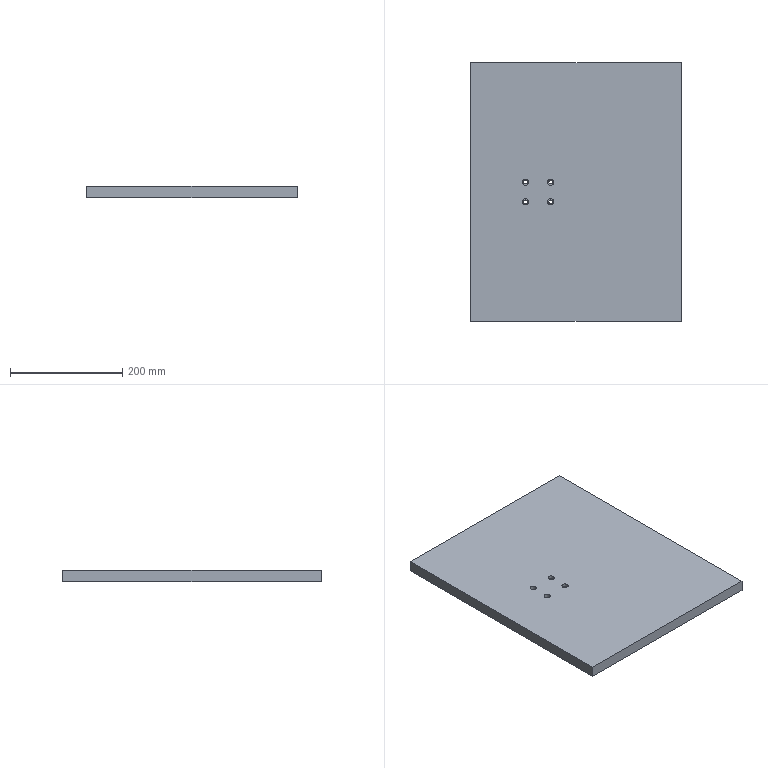Part | SolidWorks | features Extrusion 1, HoleWzd 1 | 1 solid | 26 faces | box 375 x 460 x 20 mm | volume 3445803 mm3 | cylinder 16 | plane 10 | commonest cylinder face diameters 6.6 x8 11 x8
STEP:
#1=CARTESIAN_POINT('',(-28.,247.5,14.));
#2=VERTEX_POINT('',#1);
#3=CARTESIAN_POINT('',(-17.,247.5,14.));
#4=VERTEX_POINT('',#3);
#5=CARTESIAN_POINT('',(-22.5,247.5,14.));
#6=DIRECTION('',(0.,0.,1.));
#7=DIRECTION('',(1.,0.,0.));
#8=AXIS2_PLACEMENT_3D('',#5,#6,#7);
#9=CIRCLE('',#8,5.5);
#10=EDGE_CURVE('',#2,#4,#9,.T.);
#11=ORIENTED_EDGE('',*,*,#10,.F.);
#12=CARTESIAN_POINT('',(-28.,247.5,20.));
#13=VERTEX_POINT('',#12);
#14=CARTESIAN_POINT('',(-28.,247.5,20.));
#15=DIRECTION('',(0.,0.,1.));
#16=VECTOR('',#15,1000.);
#17=LINE('',#14,#16);
#18=EDGE_CURVE('',#2,#13,#17,.T.);
#19=ORIENTED_EDGE('',*,*,#18,.T.);
#20=CARTESIAN_POINT('',(-17.,247.5,20.));
#21=VERTEX_POINT('',#20);
#22=CARTESIAN_POINT('',(-22.5,247.5,20.));
#23=DIRECTION('',(0.,0.,1.));
#24=DIRECTION('',(1.,0.,0.));
#25=AXIS2_PLACEMENT_3D('',#22,#23,#24);
#26=CIRCLE('',#25,5.5);
#27=EDGE_CURVE('',#13,#21,#26,.T.);
#28=ORIENTED_EDGE('',*,*,#27,.T.);
#29=CARTESIAN_POINT('',(-17.,247.5,20.));
#30=DIRECTION('',(0.,0.,1.));
#31=VECTOR('',#30,1000.);
#32=LINE('',#29,#31);
#33=EDGE_CURVE('',#4,#21,#32,.T.);
#34=ORIENTED_EDGE('',*,*,#33,.F.);
#35=EDGE_LOOP('',(#11,#19,#28,#34));
#36=FACE_OUTER_BOUND('',#35,.T.);
#37=CARTESIAN_POINT('',(-22.5,247.5,20.));
#38=DIRECTION('',(0.,0.,1.));
#39=DIRECTION('',(1.,0.,0.));
#40=AXIS2_PLACEMENT_3D('',#37,#38,#39);
#41=CYLINDRICAL_SURFACE('',#40,5.5);
#42=ADVANCED_FACE('',(#36),#41,.F.);
#43=CARTESIAN_POINT('',(-25.8,247.5,0.));
#44=VERTEX_POINT('',#43);
#45=CARTESIAN_POINT('',(-19.2,247.5,0.));
#46=VERTEX_POINT('',#45);
#47=CARTESIAN_POINT('',(-22.5,247.5,0.));
#48=DIRECTION('',(0.,0.,1.));
#49=DIRECTION('',(1.,0.,0.));
#50=AXIS2_PLACEMENT_3D('',#47,#48,#49);
#51=CIRCLE('',#50,3.3);
#52=EDGE_CURVE('',#44,#46,#51,.T.);
#53=ORIENTED_EDGE('',*,*,#52,.F.);
#54=CARTESIAN_POINT('',(-25.8,247.5,14.));
#55=VERTEX_POINT('',#54);
#56=CARTESIAN_POINT('',(-25.8,247.5,20.));
#57=DIRECTION('',(0.,0.,1.));
#58=VECTOR('',#57,1000.);
#59=LINE('',#56,#58);
#60=EDGE_CURVE('',#44,#55,#59,.T.);
#61=ORIENTED_EDGE('',*,*,#60,.T.);
#62=CARTESIAN_POINT('',(-19.2,247.5,14.));
#63=VERTEX_POINT('',#62);
#64=CARTESIAN_POINT('',(-22.5,247.5,14.));
#65=DIRECTION('',(0.,0.,1.));
#66=DIRECTION('',(1.,0.,0.));
#67=AXIS2_PLACEMENT_3D('',#64,#65,#66);
#68=CIRCLE('',#67,3.3);
#69=EDGE_CURVE('',#55,#63,#68,.T.);
#70=ORIENTED_EDGE('',*,*,#69,.T.);
#71=CARTESIAN_POINT('',(-19.2,247.5,20.));
#72=DIRECTION('',(0.,0.,1.));
#73=VECTOR('',#72,1000.);
#74=LINE('',#71,#73);
#75=EDGE_CURVE('',#46,#63,#74,.T.);
#76=ORIENTED_EDGE('',*,*,#75,.F.);
#77=EDGE_LOOP('',(#53,#61,#70,#76));
#78=FACE_OUTER_BOUND('',#77,.T.);
#79=CARTESIAN_POINT('',(-22.5,247.5,20.));
#80=DIRECTION('',(0.,0.,1.));
#81=DIRECTION('',(1.,0.,0.));
#82=AXIS2_PLACEMENT_3D('',#79,#80,#81);
#83=CYLINDRICAL_SURFACE('',#82,3.3);
#84=ADVANCED_FACE('',(#78),#83,.F.);
#85=CARTESIAN_POINT('',(17.,247.5,14.));
#86=VERTEX_POINT('',#85);
#87=CARTESIAN_POINT('',(28.,247.5,14.));
#88=VERTEX_POINT('',#87);
#89=CARTESIAN_POINT('',(22.5,247.5,14.));
#90=DIRECTION('',(0.,0.,1.));
#91=DIRECTION('',(1.,0.,0.));
#92=AXIS2_PLACEMENT_3D('',#89,#90,#91);
#93=CIRCLE('',#92,5.5);
#94=EDGE_CURVE('',#86,#88,#93,.T.);
#95=ORIENTED_EDGE('',*,*,#94,.F.);
#96=CARTESIAN_POINT('',(17.,247.5,20.));
#97=VERTEX_POINT('',#96);
#98=CARTESIAN_POINT('',(17.,247.5,20.));
#99=DIRECTION('',(0.,0.,1.));
#100=VECTOR('',#99,1000.);
#101=LINE('',#98,#100);
#102=EDGE_CURVE('',#86,#97,#101,.T.);
#103=ORIENTED_EDGE('',*,*,#102,.T.);
#104=CARTESIAN_POINT('',(28.,247.5,20.));
#105=VERTEX_POINT('',#104);
#106=CARTESIAN_POINT('',(22.5,247.5,20.));
#107=DIRECTION('',(0.,0.,1.));
#108=DIRECTION('',(1.,0.,0.));
#109=AXIS2_PLACEMENT_3D('',#106,#107,#108);
#110=CIRCLE('',#109,5.5);
#111=EDGE_CURVE('',#97,#105,#110,.T.);
#112=ORIENTED_EDGE('',*,*,#111,.T.);
#113=CARTESIAN_POINT('',(28.,247.5,20.));
#114=DIRECTION('',(0.,0.,1.));
#115=VECTOR('',#114,1000.);
#116=LINE('',#113,#115);
#117=EDGE_CURVE('',#88,#105,#116,.T.);
#118=ORIENTED_EDGE('',*,*,#117,.F.);
#119=EDGE_LOOP('',(#95,#103,#112,#118));
#120=FACE_OUTER_BOUND('',#119,.T.);
#121=CARTESIAN_POINT('',(22.5,247.5,20.));
#122=DIRECTION('',(0.,0.,1.));
#123=DIRECTION('',(1.,0.,0.));
#124=AXIS2_PLACEMENT_3D('',#121,#122,#123);
#125=CYLINDRICAL_SURFACE('',#124,5.5);
#126=ADVANCED_FACE('',(#120),#125,.F.);
#127=CARTESIAN_POINT('',(19.2,247.5,0.));
#128=VERTEX_POINT('',#127);
#129=CARTESIAN_POINT('',(25.8,247.5,0.));
#130=VERTEX_POINT('',#129);
#131=CARTESIAN_POINT('',(22.5,247.5,0.));
#132=DIRECTION('',(0.,0.,1.));
#133=DIRECTION('',(1.,0.,0.));
#134=AXIS2_PLACEMENT_3D('',#131,#132,#133);
#135=CIRCLE('',#134,3.3);
#136=EDGE_CURVE('',#128,#130,#135,.T.);
#137=ORIENTED_EDGE('',*,*,#136,.F.);
#138=CARTESIAN_POINT('',(19.2,247.5,14.));
#139=VERTEX_POINT('',#138);
#140=CARTESIAN_POINT('',(19.2,247.5,20.));
#141=DIRECTION('',(0.,0.,1.));
#142=VECTOR('',#141,1000.);
#143=LINE('',#140,#142);
#144=EDGE_CURVE('',#128,#139,#143,.T.);
#145=ORIENTED_EDGE('',*,*,#144,.T.);
#146=CARTESIAN_POINT('',(25.8,247.5,14.));
#147=VERTEX_POINT('',#146);
#148=CARTESIAN_POINT('',(22.5,247.5,14.));
#149=DIRECTION('',(0.,0.,1.));
#150=DIRECTION('',(1.,0.,0.));
#151=AXIS2_PLACEMENT_3D('',#148,#149,#150);
#152=CIRCLE('',#151,3.3);
#153=EDGE_CURVE('',#139,#147,#152,.T.);
#154=ORIENTED_EDGE('',*,*,#153,.T.);
#155=CARTESIAN_POINT('',(25.8,247.5,20.));
#156=DIRECTION('',(0.,0.,1.));
#157=VECTOR('',#156,1000.);
#158=LINE('',#155,#157);
#159=EDGE_CURVE('',#130,#147,#158,.T.);
#160=ORIENTED_EDGE('',*,*,#159,.F.);
#161=EDGE_LOOP('',(#137,#145,#154,#160));
#162=FACE_OUTER_BOUND('',#161,.T.);
#163=CARTESIAN_POINT('',(22.5,247.5,20.));
#164=DIRECTION('',(0.,0.,1.));
#165=DIRECTION('',(1.,0.,0.));
#166=AXIS2_PLACEMENT_3D('',#163,#164,#165);
#167=CYLINDRICAL_SURFACE('',#166,3.3);
#168=ADVANCED_FACE('',(#162),#167,.F.);
#169=CARTESIAN_POINT('',(17.,212.5,14.));
#170=VERTEX_POINT('',#169);
#171=CARTESIAN_POINT('',(28.,212.5,14.));
#172=VERTEX_POINT('',#171);
#173=CARTESIAN_POINT('',(22.5,212.5,14.));
#174=DIRECTION('',(0.,0.,1.));
#175=DIRECTION('',(1.,0.,0.));
#176=AXIS2_PLACEMENT_3D('',#173,#174,#175);
#177=CIRCLE('',#176,5.5);
#178=EDGE_CURVE('',#170,#172,#177,.T.);
#179=ORIENTED_EDGE('',*,*,#178,.F.);
#180=CARTESIAN_POINT('',(17.,212.5,20.));
#181=VERTEX_POINT('',#180);
#182=CARTESIAN_POINT('',(17.,212.5,20.));
#183=DIRECTION('',(0.,0.,1.));
#184=VECTOR('',#183,1000.);
#185=LINE('',#182,#184);
#186=EDGE_CURVE('',#170,#181,#185,.T.);
#187=ORIENTED_EDGE('',*,*,#186,.T.);
#188=CARTESIAN_POINT('',(28.,212.5,20.));
#189=VERTEX_POINT('',#188);
#190=CARTESIAN_POINT('',(22.5,212.5,20.));
#191=DIRECTION('',(0.,0.,1.));
#192=DIRECTION('',(1.,0.,0.));
#193=AXIS2_PLACEMENT_3D('',#190,#191,#192);
#194=CIRCLE('',#193,5.5);
#195=EDGE_CURVE('',#181,#189,#194,.T.);
#196=ORIENTED_EDGE('',*,*,#195,.T.);
#197=CARTESIAN_POINT('',(28.,212.5,20.));
#198=DIRECTION('',(0.,0.,1.));
#199=VECTOR('',#198,1000.);
#200=LINE('',#197,#199);
#201=EDGE_CURVE('',#172,#189,#200,.T.);
#202=ORIENTED_EDGE('',*,*,#201,.F.);
#203=EDGE_LOOP('',(#179,#187,#196,#202));
#204=FACE_OUTER_BOUND('',#203,.T.);
#205=CARTESIAN_POINT('',(22.5,212.5,20.));
#206=DIRECTION('',(0.,0.,1.));
#207=DIRECTION('',(1.,0.,0.));
#208=AXIS2_PLACEMENT_3D('',#205,#206,#207);
#209=CYLINDRICAL_SURFACE('',#208,5.5);
#210=ADVANCED_FACE('',(#204),#209,.F.);
#211=CARTESIAN_POINT('',(19.2,212.5,0.));
#212=VERTEX_POINT('',#211);
#213=CARTESIAN_POINT('',(25.8,212.5,0.));
#214=VERTEX_POINT('',#213);
#215=CARTESIAN_POINT('',(22.5,212.5,0.));
#216=DIRECTION('',(0.,0.,1.));
#217=DIRECTION('',(1.,0.,0.));
#218=AXIS2_PLACEMENT_3D('',#215,#216,#217);
#219=CIRCLE('',#218,3.3);
#220=EDGE_CURVE('',#212,#214,#219,.T.);
#221=ORIENTED_EDGE('',*,*,#220,.F.);
#222=CARTESIAN_POINT('',(19.2,212.5,14.));
#223=VERTEX_POINT('',#222);
#224=CARTESIAN_POINT('',(19.2,212.5,20.));
#225=DIRECTION('',(0.,0.,1.));
#226=VECTOR('',#225,1000.);
#227=LINE('',#224,#226);
#228=EDGE_CURVE('',#212,#223,#227,.T.);
#229=ORIENTED_EDGE('',*,*,#228,.T.);
#230=CARTESIAN_POINT('',(25.8,212.5,14.));
#231=VERTEX_POINT('',#230);
#232=CARTESIAN_POINT('',(22.5,212.5,14.));
#233=DIRECTION('',(0.,0.,1.));
#234=DIRECTION('',(1.,0.,0.));
#235=AXIS2_PLACEMENT_3D('',#232,#233,#234);
#236=CIRCLE('',#235,3.3);
#237=EDGE_CURVE('',#223,#231,#236,.T.);
#238=ORIENTED_EDGE('',*,*,#237,.T.);
#239=CARTESIAN_POINT('',(25.8,212.5,20.));
#240=DIRECTION('',(0.,0.,1.));
#241=VECTOR('',#240,1000.);
#242=LINE('',#239,#241);
#243=EDGE_CURVE('',#214,#231,#242,.T.);
#244=ORIENTED_EDGE('',*,*,#243,.F.);
#245=EDGE_LOOP('',(#221,#229,#238,#244));
#246=FACE_OUTER_BOUND('',#245,.T.);
#247=CARTESIAN_POINT('',(22.5,212.5,20.));
#248=DIRECTION('',(0.,0.,1.));
#249=DIRECTION('',(1.,0.,0.));
#250=AXIS2_PLACEMENT_3D('',#247,#248,#249);
#251=CYLINDRICAL_SURFACE('',#250,3.3);
#252=ADVANCED_FACE('',(#246),#251,.F.);
#253=CARTESIAN_POINT('',(-28.,212.5,14.));
#254=VERTEX_POINT('',#253);
#255=CARTESIAN_POINT('',(-17.,212.5,14.));
#256=VERTEX_POINT('',#255);
#257=CARTESIAN_POINT('',(-22.5,212.5,14.));
#258=DIRECTION('',(0.,0.,1.));
#259=DIRECTION('',(1.,0.,0.));
#260=AXIS2_PLACEMENT_3D('',#257,#258,#259);
#261=CIRCLE('',#260,5.5);
#262=EDGE_CURVE('',#254,#256,#261,.T.);
#263=ORIENTED_EDGE('',*,*,#262,.F.);
#264=CARTESIAN_POINT('',(-28.,212.5,20.));
#265=VERTEX_POINT('',#264);
#266=CARTESIAN_POINT('',(-28.,212.5,20.));
#267=DIRECTION('',(0.,0.,1.));
#268=VECTOR('',#267,1000.);
#269=LINE('',#266,#268);
#270=EDGE_CURVE('',#254,#265,#269,.T.);
#271=ORIENTED_EDGE('',*,*,#270,.T.);
#272=CARTESIAN_POINT('',(-17.,212.5,20.));
#273=VERTEX_POINT('',#272);
#274=CARTESIAN_POINT('',(-22.5,212.5,20.));
#275=DIRECTION('',(0.,0.,1.));
#276=DIRECTION('',(1.,0.,0.));
#277=AXIS2_PLACEMENT_3D('',#274,#275,#276);
#278=CIRCLE('',#277,5.5);
#279=EDGE_CURVE('',#265,#273,#278,.T.);
#280=ORIENTED_EDGE('',*,*,#279,.T.);
#281=CARTESIAN_POINT('',(-17.,212.5,20.));
#282=DIRECTION('',(0.,0.,1.));
#283=VECTOR('',#282,1000.);
#284=LINE('',#281,#283);
#285=EDGE_CURVE('',#256,#273,#284,.T.);
#286=ORIENTED_EDGE('',*,*,#285,.F.);
#287=EDGE_LOOP('',(#263,#271,#280,#286));
#288=FACE_OUTER_BOUND('',#287,.T.);
#289=CARTESIAN_POINT('',(-22.5,212.5,20.));
#290=DIRECTION('',(0.,0.,1.));
#291=DIRECTION('',(1.,0.,0.));
#292=AXIS2_PLACEMENT_3D('',#289,#290,#291);
#293=CYLINDRICAL_SURFACE('',#292,5.5);
#294=ADVANCED_FACE('',(#288),#293,.F.);
#295=CARTESIAN_POINT('',(-25.8,212.5,0.));
#296=VERTEX_POINT('',#295);
#297=CARTESIAN_POINT('',(-19.2,212.5,0.));
#298=VERTEX_POINT('',#297);
#299=CARTESIAN_POINT('',(-22.5,212.5,0.));
#300=DIRECTION('',(0.,0.,1.));
#301=DIRECTION('',(1.,0.,0.));
#302=AXIS2_PLACEMENT_3D('',#299,#300,#301);
#303=CIRCLE('',#302,3.3);
#304=EDGE_CURVE('',#296,#298,#303,.T.);
#305=ORIENTED_EDGE('',*,*,#304,.F.);
#306=CARTESIAN_POINT('',(-25.8,212.5,14.));
#307=VERTEX_POINT('',#306);
#308=CARTESIAN_POINT('',(-25.8,212.5,20.));
#309=DIRECTION('',(0.,0.,1.));
#310=VECTOR('',#309,1000.);
#311=LINE('',#308,#310);
#312=EDGE_CURVE('',#296,#307,#311,.T.);
#313=ORIENTED_EDGE('',*,*,#312,.T.);
#314=CARTESIAN_POINT('',(-19.2,212.5,14.));
#315=VERTEX_POINT('',#314);
#316=CARTESIAN_POINT('',(-22.5,212.5,14.));
#317=DIRECTION('',(0.,0.,1.));
#318=DIRECTION('',(1.,0.,0.));
#319=AXIS2_PLACEMENT_3D('',#316,#317,#318);
#320=CIRCLE('',#319,3.3);
#321=EDGE_CURVE('',#307,#315,#320,.T.);
#322=ORIENTED_EDGE('',*,*,#321,.T.);
#323=CARTESIAN_POINT('',(-19.2,212.5,20.));
#324=DIRECTION('',(0.,0.,1.));
#325=VECTOR('',#324,1000.);
#326=LINE('',#323,#325);
#327=EDGE_CURVE('',#298,#315,#326,.T.);
#328=ORIENTED_EDGE('',*,*,#327,.F.);
#329=EDGE_LOOP('',(#305,#313,#322,#328));
#330=FACE_OUTER_BOUND('',#329,.T.);
#331=CARTESIAN_POINT('',(-22.5,212.5,20.));
#332=DIRECTION('',(0.,0.,1.));
#333=DIRECTION('',(1.,0.,0.));
#334=AXIS2_PLACEMENT_3D('',#331,#332,#333);
#335=CYLINDRICAL_SURFACE('',#334,3.3);
#336=ADVANCED_FACE('',(#330),#335,.F.);
#337=CARTESIAN_POINT('',(-120.,460.,0.));
#338=VERTEX_POINT('',#337);
#339=CARTESIAN_POINT('',(-120.,0.,0.));
#340=VERTEX_POINT('',#339);
#341=CARTESIAN_POINT('',(-120.,460.,0.));
#342=DIRECTION('',(0.,-1.,0.));
#343=VECTOR('',#342,1000.);
#344=LINE('',#341,#343);
#345=EDGE_CURVE('',#338,#340,#344,.T.);
#346=ORIENTED_EDGE('',*,*,#345,.T.);
#347=CARTESIAN_POINT('',(-120.,0.,20.));
#348=VERTEX_POINT('',#347);
#349=CARTESIAN_POINT('',(-120.,0.,20.));
#350=DIRECTION('',(0.,0.,-1.));
#351=VECTOR('',#350,1000.);
#352=LINE('',#349,#351);
#353=EDGE_CURVE('',#348,#340,#352,.T.);
#354=ORIENTED_EDGE('',*,*,#353,.F.);
#355=CARTESIAN_POINT('',(-120.,460.,20.));
#356=VERTEX_POINT('',#355);
#357=CARTESIAN_POINT('',(-120.,460.,20.));
#358=DIRECTION('',(0.,-1.,0.));
#359=VECTOR('',#358,1000.);
#360=LINE('',#357,#359);
#361=EDGE_CURVE('',#356,#348,#360,.T.);
#362=ORIENTED_EDGE('',*,*,#361,.F.);
#363=CARTESIAN_POINT('',(-120.,460.,20.));
#364=DIRECTION('',(0.,0.,-1.));
#365=VECTOR('',#364,1000.);
#366=LINE('',#363,#365);
#367=EDGE_CURVE('',#356,#338,#366,.T.);
#368=ORIENTED_EDGE('',*,*,#367,.T.);
#369=EDGE_LOOP('',(#346,#354,#362,#368));
#370=FACE_OUTER_BOUND('',#369,.T.);
#371=CARTESIAN_POINT('',(-120.,460.,20.));
#372=DIRECTION('',(1.,0.,0.));
#373=DIRECTION('',(0.,0.,-1.));
#374=AXIS2_PLACEMENT_3D('',#371,#372,#373);
#375=PLANE('',#374);
#376=ADVANCED_FACE('',(#370),#375,.F.);
#377=CARTESIAN_POINT('',(255.,0.,0.));
#378=VERTEX_POINT('',#377);
#379=CARTESIAN_POINT('',(-120.,0.,0.));
#380=DIRECTION('',(1.,0.,0.));
#381=VECTOR('',#380,1000.);
#382=LINE('',#379,#381);
#383=EDGE_CURVE('',#340,#378,#382,.T.);
#384=ORIENTED_EDGE('',*,*,#383,.T.);
#385=CARTESIAN_POINT('',(255.,0.,20.));
#386=VERTEX_POINT('',#385);
#387=CARTESIAN_POINT('',(255.,0.,20.));
#388=DIRECTION('',(0.,0.,-1.));
#389=VECTOR('',#388,1000.);
#390=LINE('',#387,#389);
#391=EDGE_CURVE('',#386,#378,#390,.T.);
#392=ORIENTED_EDGE('',*,*,#391,.F.);
#393=CARTESIAN_POINT('',(-120.,0.,20.));
#394=DIRECTION('',(1.,0.,0.));
#395=VECTOR('',#394,1000.);
#396=LINE('',#393,#395);
#397=EDGE_CURVE('',#348,#386,#396,.T.);
#398=ORIENTED_EDGE('',*,*,#397,.F.);
#399=ORIENTED_EDGE('',*,*,#353,.T.);
#400=EDGE_LOOP('',(#384,#392,#398,#399));
#401=FACE_OUTER_BOUND('',#400,.T.);
#402=CARTESIAN_POINT('',(-120.,0.,20.));
#403=DIRECTION('',(0.,1.,0.));
#404=DIRECTION('',(-1.,0.,0.));
#405=AXIS2_PLACEMENT_3D('',#402,#403,#404);
#406=PLANE('',#405);
#407=ADVANCED_FACE('',(#401),#406,.F.);
#408=CARTESIAN_POINT('',(255.,460.,0.));
#409=VERTEX_POINT('',#408);
#410=CARTESIAN_POINT('',(255.,460.,0.));
#411=DIRECTION('',(0.,-1.,0.));
#412=VECTOR('',#411,1000.);
#413=LINE('',#410,#412);
#414=EDGE_CURVE('',#409,#378,#413,.T.);
#415=ORIENTED_EDGE('',*,*,#414,.F.);
#416=CARTESIAN_POINT('',(255.,460.,20.));
#417=VERTEX_POINT('',#416);
#418=CARTESIAN_POINT('',(255.,460.,20.));
#419=DIRECTION('',(0.,0.,-1.));
#420=VECTOR('',#419,1000.);
#421=LINE('',#418,#420);
#422=EDGE_CURVE('',#417,#409,#421,.T.);
#423=ORIENTED_EDGE('',*,*,#422,.F.);
#424=CARTESIAN_POINT('',(255.,460.,20.));
#425=DIRECTION('',(0.,-1.,0.));
#426=VECTOR('',#425,1000.);
#427=LINE('',#424,#426);
#428=EDGE_CURVE('',#417,#386,#427,.T.);
#429=ORIENTED_EDGE('',*,*,#428,.T.);
#430=ORIENTED_EDGE('',*,*,#391,.T.);
#431=EDGE_LOOP('',(#415,#423,#429,#430));
#432=FACE_OUTER_BOUND('',#431,.T.);
#433=CARTESIAN_POINT('',(255.,460.,20.));
#434=DIRECTION('',(1.,0.,0.));
#435=DIRECTION('',(0.,1.,0.));
#436=AXIS2_PLACEMENT_3D('',#433,#434,#435);
#437=PLANE('',#436);
#438=ADVANCED_FACE('',(#432),#437,.T.);
#439=CARTESIAN_POINT('',(-120.,460.,0.));
#440=DIRECTION('',(1.,0.,0.));
#441=VECTOR('',#440,1000.);
#442=LINE('',#439,#441);
#443=EDGE_CURVE('',#338,#409,#442,.T.);
#444=ORIENTED_EDGE('',*,*,#443,.F.);
#445=ORIENTED_EDGE('',*,*,#367,.F.);
#446=CARTESIAN_POINT('',(-120.,460.,20.));
#447=DIRECTION('',(1.,0.,0.));
#448=VECTOR('',#447,1000.);
#449=LINE('',#446,#448);
#450=EDGE_CURVE('',#356,#417,#449,.T.);
#451=ORIENTED_EDGE('',*,*,#450,.T.);
#452=ORIENTED_EDGE('',*,*,#422,.T.);
#453=EDGE_LOOP('',(#444,#445,#451,#452));
#454=FACE_OUTER_BOUND('',#453,.T.);
#455=CARTESIAN_POINT('',(-120.,460.,20.));
#456=DIRECTION('',(0.,1.,0.));
#457=DIRECTION('',(0.,0.,1.));
#458=AXIS2_PLACEMENT_3D('',#455,#456,#457);
#459=PLANE('',#458);
#460=ADVANCED_FACE('',(#454),#459,.T.);
#461=CARTESIAN_POINT('',(-22.5,247.5,20.));
#462=DIRECTION('',(0.,0.,1.));
#463=DIRECTION('',(1.,0.,0.));
#464=AXIS2_PLACEMENT_3D('',#461,#462,#463);
#465=CIRCLE('',#464,5.5);
#466=EDGE_CURVE('',#21,#13,#465,.T.);
#467=ORIENTED_EDGE('',*,*,#466,.F.);
#468=ORIENTED_EDGE('',*,*,#27,.F.);
#469=EDGE_LOOP('',(#467,#468));
#470=FACE_BOUND('',#469,.T.);
#471=CARTESIAN_POINT('',(22.5,247.5,20.));
#472=DIRECTION('',(0.,0.,1.));
#473=DIRECTION('',(1.,0.,0.));
#474=AXIS2_PLACEMENT_3D('',#471,#472,#473);
#475=CIRCLE('',#474,5.5);
#476=EDGE_CURVE('',#105,#97,#475,.T.);
#477=ORIENTED_EDGE('',*,*,#476,.F.);
#478=ORIENTED_EDGE('',*,*,#111,.F.);
#479=EDGE_LOOP('',(#477,#478));
#480=FACE_BOUND('',#479,.T.);
#481=CARTESIAN_POINT('',(22.5,212.5,20.));
#482=DIRECTION('',(0.,0.,1.));
#483=DIRECTION('',(1.,0.,0.));
#484=AXIS2_PLACEMENT_3D('',#481,#482,#483);
#485=CIRCLE('',#484,5.5);
#486=EDGE_CURVE('',#189,#181,#485,.T.);
#487=ORIENTED_EDGE('',*,*,#486,.F.);
#488=ORIENTED_EDGE('',*,*,#195,.F.);
#489=EDGE_LOOP('',(#487,#488));
#490=FACE_BOUND('',#489,.T.);
#491=CARTESIAN_POINT('',(-22.5,212.5,20.));
#492=DIRECTION('',(0.,0.,1.));
#493=DIRECTION('',(1.,0.,0.));
#494=AXIS2_PLACEMENT_3D('',#491,#492,#493);
#495=CIRCLE('',#494,5.5);
#496=EDGE_CURVE('',#273,#265,#495,.T.);
#497=ORIENTED_EDGE('',*,*,#496,.F.);
#498=ORIENTED_EDGE('',*,*,#279,.F.);
#499=EDGE_LOOP('',(#497,#498));
#500=FACE_BOUND('',#499,.T.);
#501=ORIENTED_EDGE('',*,*,#361,.T.);
#502=ORIENTED_EDGE('',*,*,#397,.T.);
#503=ORIENTED_EDGE('',*,*,#428,.F.);
#504=ORIENTED_EDGE('',*,*,#450,.F.);
#505=EDGE_LOOP('',(#501,#502,#503,#504));
#506=FACE_OUTER_BOUND('',#505,.T.);
#507=CARTESIAN_POINT('',(0.,0.,20.));
#508=DIRECTION('',(0.,0.,1.));
#509=DIRECTION('',(1.,0.,0.));
#510=AXIS2_PLACEMENT_3D('',#507,#508,#509);
#511=PLANE('',#510);
#512=ADVANCED_FACE('',(#470,#480,#490,#500,#506),#511,.T.);
#513=CARTESIAN_POINT('',(-22.5,247.5,0.));
#514=DIRECTION('',(0.,0.,1.));
#515=DIRECTION('',(1.,0.,0.));
#516=AXIS2_PLACEMENT_3D('',#513,#514,#515);
#517=CIRCLE('',#516,3.3);
#518=EDGE_CURVE('',#46,#44,#517,.T.);
#519=ORIENTED_EDGE('',*,*,#518,.T.);
#520=ORIENTED_EDGE('',*,*,#52,.T.);
#521=EDGE_LOOP('',(#519,#520));
#522=FACE_BOUND('',#521,.T.);
#523=CARTESIAN_POINT('',(22.5,247.5,0.));
#524=DIRECTION('',(0.,0.,1.));
#525=DIRECTION('',(1.,0.,0.));
#526=AXIS2_PLACEMENT_3D('',#523,#524,#525);
#527=CIRCLE('',#526,3.3);
#528=EDGE_CURVE('',#130,#128,#527,.T.);
#529=ORIENTED_EDGE('',*,*,#528,.T.);
#530=ORIENTED_EDGE('',*,*,#136,.T.);
#531=EDGE_LOOP('',(#529,#530));
#532=FACE_BOUND('',#531,.T.);
#533=CARTESIAN_POINT('',(22.5,212.5,0.));
#534=DIRECTION('',(0.,0.,1.));
#535=DIRECTION('',(1.,0.,0.));
#536=AXIS2_PLACEMENT_3D('',#533,#534,#535);
#537=CIRCLE('',#536,3.3);
#538=EDGE_CURVE('',#214,#212,#537,.T.);
#539=ORIENTED_EDGE('',*,*,#538,.T.);
#540=ORIENTED_EDGE('',*,*,#220,.T.);
#541=EDGE_LOOP('',(#539,#540));
#542=FACE_BOUND('',#541,.T.);
#543=CARTESIAN_POINT('',(-22.5,212.5,0.));
#544=DIRECTION('',(0.,0.,1.));
#545=DIRECTION('',(1.,0.,0.));
#546=AXIS2_PLACEMENT_3D('',#543,#544,#545);
#547=CIRCLE('',#546,3.3);
#548=EDGE_CURVE('',#298,#296,#547,.T.);
#549=ORIENTED_EDGE('',*,*,#548,.T.);
#550=ORIENTED_EDGE('',*,*,#304,.T.);
#551=EDGE_LOOP('',(#549,#550));
#552=FACE_BOUND('',#551,.T.);
#553=ORIENTED_EDGE('',*,*,#345,.F.);
#554=ORIENTED_EDGE('',*,*,#443,.T.);
#555=ORIENTED_EDGE('',*,*,#414,.T.);
#556=ORIENTED_EDGE('',*,*,#383,.F.);
#557=EDGE_LOOP('',(#553,#554,#555,#556));
#558=FACE_OUTER_BOUND('',#557,.T.);
#559=CARTESIAN_POINT('',(0.,0.,0.));
#560=DIRECTION('',(0.,0.,1.));
#561=DIRECTION('',(1.,0.,0.));
#562=AXIS2_PLACEMENT_3D('',#559,#560,#561);
#563=PLANE('',#562);
#564=ADVANCED_FACE('',(#522,#532,#542,#552,#558),#563,.F.);
#565=ORIENTED_EDGE('',*,*,#312,.F.);
#566=ORIENTED_EDGE('',*,*,#548,.F.);
#567=ORIENTED_EDGE('',*,*,#327,.T.);
#568=CARTESIAN_POINT('',(-22.5,212.5,14.));
#569=DIRECTION('',(0.,0.,1.));
#570=DIRECTION('',(1.,0.,0.));
#571=AXIS2_PLACEMENT_3D('',#568,#569,#570);
#572=CIRCLE('',#571,3.3);
#573=EDGE_CURVE('',#315,#307,#572,.T.);
#574=ORIENTED_EDGE('',*,*,#573,.T.);
#575=EDGE_LOOP('',(#565,#566,#567,#574));
#576=FACE_OUTER_BOUND('',#575,.T.);
#577=CARTESIAN_POINT('',(-22.5,212.5,20.));
#578=DIRECTION('',(0.,0.,1.));
#579=DIRECTION('',(1.,0.,0.));
#580=AXIS2_PLACEMENT_3D('',#577,#578,#579);
#581=CYLINDRICAL_SURFACE('',#580,3.3);
#582=ADVANCED_FACE('',(#576),#581,.F.);
#583=ORIENTED_EDGE('',*,*,#573,.F.);
#584=ORIENTED_EDGE('',*,*,#321,.F.);
#585=EDGE_LOOP('',(#583,#584));
#586=FACE_BOUND('',#585,.T.);
#587=CARTESIAN_POINT('',(-22.5,212.5,14.));
#588=DIRECTION('',(0.,0.,1.));
#589=DIRECTION('',(1.,0.,0.));
#590=AXIS2_PLACEMENT_3D('',#587,#588,#589);
#591=CIRCLE('',#590,5.5);
#592=EDGE_CURVE('',#256,#254,#591,.T.);
#593=ORIENTED_EDGE('',*,*,#592,.T.);
#594=ORIENTED_EDGE('',*,*,#262,.T.);
#595=EDGE_LOOP('',(#593,#594));
#596=FACE_OUTER_BOUND('',#595,.T.);
#597=CARTESIAN_POINT('',(-19.2,212.5,14.));
#598=DIRECTION('',(0.,0.,-1.));
#599=DIRECTION('',(-1.,0.,0.));
#600=AXIS2_PLACEMENT_3D('',#597,#598,#599);
#601=PLANE('',#600);
#602=ADVANCED_FACE('',(#586,#596),#601,.F.);
#603=ORIENTED_EDGE('',*,*,#270,.F.);
#604=ORIENTED_EDGE('',*,*,#592,.F.);
#605=ORIENTED_EDGE('',*,*,#285,.T.);
#606=ORIENTED_EDGE('',*,*,#496,.T.);
#607=EDGE_LOOP('',(#603,#604,#605,#606));
#608=FACE_OUTER_BOUND('',#607,.T.);
#609=CARTESIAN_POINT('',(-22.5,212.5,20.));
#610=DIRECTION('',(0.,0.,1.));
#611=DIRECTION('',(1.,0.,0.));
#612=AXIS2_PLACEMENT_3D('',#609,#610,#611);
#613=CYLINDRICAL_SURFACE('',#612,5.5);
#614=ADVANCED_FACE('',(#608),#613,.F.);
#615=ORIENTED_EDGE('',*,*,#228,.F.);
#616=ORIENTED_EDGE('',*,*,#538,.F.);
#617=ORIENTED_EDGE('',*,*,#243,.T.);
#618=CARTESIAN_POINT('',(22.5,212.5,14.));
#619=DIRECTION('',(0.,0.,1.));
#620=DIRECTION('',(1.,0.,0.));
#621=AXIS2_PLACEMENT_3D('',#618,#619,#620);
#622=CIRCLE('',#621,3.3);
#623=EDGE_CURVE('',#231,#223,#622,.T.);
#624=ORIENTED_EDGE('',*,*,#623,.T.);
#625=EDGE_LOOP('',(#615,#616,#617,#624));
#626=FACE_OUTER_BOUND('',#625,.T.);
#627=CARTESIAN_POINT('',(22.5,212.5,20.));
#628=DIRECTION('',(0.,0.,1.));
#629=DIRECTION('',(1.,0.,0.));
#630=AXIS2_PLACEMENT_3D('',#627,#628,#629);
#631=CYLINDRICAL_SURFACE('',#630,3.3);
#632=ADVANCED_FACE('',(#626),#631,.F.);
#633=ORIENTED_EDGE('',*,*,#623,.F.);
#634=ORIENTED_EDGE('',*,*,#237,.F.);
#635=EDGE_LOOP('',(#633,#634));
#636=FACE_BOUND('',#635,.T.);
#637=CARTESIAN_POINT('',(22.5,212.5,14.));
#638=DIRECTION('',(0.,0.,1.));
#639=DIRECTION('',(1.,0.,0.));
#640=AXIS2_PLACEMENT_3D('',#637,#638,#639);
#641=CIRCLE('',#640,5.5);
#642=EDGE_CURVE('',#172,#170,#641,.T.);
#643=ORIENTED_EDGE('',*,*,#642,.T.);
#644=ORIENTED_EDGE('',*,*,#178,.T.);
#645=EDGE_LOOP('',(#643,#644));
#646=FACE_OUTER_BOUND('',#645,.T.);
#647=CARTESIAN_POINT('',(25.8,212.5,14.));
#648=DIRECTION('',(0.,0.,-1.));
#649=DIRECTION('',(-1.,0.,0.));
#650=AXIS2_PLACEMENT_3D('',#647,#648,#649);
#651=PLANE('',#650);
#652=ADVANCED_FACE('',(#636,#646),#651,.F.);
#653=ORIENTED_EDGE('',*,*,#186,.F.);
#654=ORIENTED_EDGE('',*,*,#642,.F.);
#655=ORIENTED_EDGE('',*,*,#201,.T.);
#656=ORIENTED_EDGE('',*,*,#486,.T.);
#657=EDGE_LOOP('',(#653,#654,#655,#656));
#658=FACE_OUTER_BOUND('',#657,.T.);
#659=CARTESIAN_POINT('',(22.5,212.5,20.));
#660=DIRECTION('',(0.,0.,1.));
#661=DIRECTION('',(1.,0.,0.));
#662=AXIS2_PLACEMENT_3D('',#659,#660,#661);
#663=CYLINDRICAL_SURFACE('',#662,5.5);
#664=ADVANCED_FACE('',(#658),#663,.F.);
#665=ORIENTED_EDGE('',*,*,#144,.F.);
#666=ORIENTED_EDGE('',*,*,#528,.F.);
#667=ORIENTED_EDGE('',*,*,#159,.T.);
#668=CARTESIAN_POINT('',(22.5,247.5,14.));
#669=DIRECTION('',(0.,0.,1.));
#670=DIRECTION('',(1.,0.,0.));
#671=AXIS2_PLACEMENT_3D('',#668,#669,#670);
#672=CIRCLE('',#671,3.3);
#673=EDGE_CURVE('',#147,#139,#672,.T.);
#674=ORIENTED_EDGE('',*,*,#673,.T.);
#675=EDGE_LOOP('',(#665,#666,#667,#674));
#676=FACE_OUTER_BOUND('',#675,.T.);
#677=CARTESIAN_POINT('',(22.5,247.5,20.));
#678=DIRECTION('',(0.,0.,1.));
#679=DIRECTION('',(1.,0.,0.));
#680=AXIS2_PLACEMENT_3D('',#677,#678,#679);
#681=CYLINDRICAL_SURFACE('',#680,3.3);
#682=ADVANCED_FACE('',(#676),#681,.F.);
#683=ORIENTED_EDGE('',*,*,#673,.F.);
#684=ORIENTED_EDGE('',*,*,#153,.F.);
#685=EDGE_LOOP('',(#683,#684));
#686=FACE_BOUND('',#685,.T.);
#687=CARTESIAN_POINT('',(22.5,247.5,14.));
#688=DIRECTION('',(0.,0.,1.));
#689=DIRECTION('',(1.,0.,0.));
#690=AXIS2_PLACEMENT_3D('',#687,#688,#689);
#691=CIRCLE('',#690,5.5);
#692=EDGE_CURVE('',#88,#86,#691,.T.);
#693=ORIENTED_EDGE('',*,*,#692,.T.);
#694=ORIENTED_EDGE('',*,*,#94,.T.);
#695=EDGE_LOOP('',(#693,#694));
#696=FACE_OUTER_BOUND('',#695,.T.);
#697=CARTESIAN_POINT('',(25.8,247.5,14.));
#698=DIRECTION('',(0.,0.,-1.));
#699=DIRECTION('',(-1.,0.,0.));
#700=AXIS2_PLACEMENT_3D('',#697,#698,#699);
#701=PLANE('',#700);
#702=ADVANCED_FACE('',(#686,#696),#701,.F.);
#703=ORIENTED_EDGE('',*,*,#102,.F.);
#704=ORIENTED_EDGE('',*,*,#692,.F.);
#705=ORIENTED_EDGE('',*,*,#117,.T.);
#706=ORIENTED_EDGE('',*,*,#476,.T.);
#707=EDGE_LOOP('',(#703,#704,#705,#706));
#708=FACE_OUTER_BOUND('',#707,.T.);
#709=CARTESIAN_POINT('',(22.5,247.5,20.));
#710=DIRECTION('',(0.,0.,1.));
#711=DIRECTION('',(1.,0.,0.));
#712=AXIS2_PLACEMENT_3D('',#709,#710,#711);
#713=CYLINDRICAL_SURFACE('',#712,5.5);
#714=ADVANCED_FACE('',(#708),#713,.F.);
#715=ORIENTED_EDGE('',*,*,#60,.F.);
#716=ORIENTED_EDGE('',*,*,#518,.F.);
#717=ORIENTED_EDGE('',*,*,#75,.T.);
#718=CARTESIAN_POINT('',(-22.5,247.5,14.));
#719=DIRECTION('',(0.,0.,1.));
#720=DIRECTION('',(1.,0.,0.));
#721=AXIS2_PLACEMENT_3D('',#718,#719,#720);
#722=CIRCLE('',#721,3.3);
#723=EDGE_CURVE('',#63,#55,#722,.T.);
#724=ORIENTED_EDGE('',*,*,#723,.T.);
#725=EDGE_LOOP('',(#715,#716,#717,#724));
#726=FACE_OUTER_BOUND('',#725,.T.);
#727=CARTESIAN_POINT('',(-22.5,247.5,20.));
#728=DIRECTION('',(0.,0.,1.));
#729=DIRECTION('',(1.,0.,0.));
#730=AXIS2_PLACEMENT_3D('',#727,#728,#729);
#731=CYLINDRICAL_SURFACE('',#730,3.3);
#732=ADVANCED_FACE('',(#726),#731,.F.);
#733=ORIENTED_EDGE('',*,*,#723,.F.);
#734=ORIENTED_EDGE('',*,*,#69,.F.);
#735=EDGE_LOOP('',(#733,#734));
#736=FACE_BOUND('',#735,.T.);
#737=CARTESIAN_POINT('',(-22.5,247.5,14.));
#738=DIRECTION('',(0.,0.,1.));
#739=DIRECTION('',(1.,0.,0.));
#740=AXIS2_PLACEMENT_3D('',#737,#738,#739);
#741=CIRCLE('',#740,5.5);
#742=EDGE_CURVE('',#4,#2,#741,.T.);
#743=ORIENTED_EDGE('',*,*,#742,.T.);
#744=ORIENTED_EDGE('',*,*,#10,.T.);
#745=EDGE_LOOP('',(#743,#744));
#746=FACE_OUTER_BOUND('',#745,.T.);
#747=CARTESIAN_POINT('',(-19.2,247.5,14.));
#748=DIRECTION('',(0.,0.,-1.));
#749=DIRECTION('',(-1.,0.,0.));
#750=AXIS2_PLACEMENT_3D('',#747,#748,#749);
#751=PLANE('',#750);
#752=ADVANCED_FACE('',(#736,#746),#751,.F.);
#753=ORIENTED_EDGE('',*,*,#18,.F.);
#754=ORIENTED_EDGE('',*,*,#742,.F.);
#755=ORIENTED_EDGE('',*,*,#33,.T.);
#756=ORIENTED_EDGE('',*,*,#466,.T.);
#757=EDGE_LOOP('',(#753,#754,#755,#756));
#758=FACE_OUTER_BOUND('',#757,.T.);
#759=CARTESIAN_POINT('',(-22.5,247.5,20.));
#760=DIRECTION('',(0.,0.,1.));
#761=DIRECTION('',(1.,0.,0.));
#762=AXIS2_PLACEMENT_3D('',#759,#760,#761);
#763=CYLINDRICAL_SURFACE('',#762,5.5);
#764=ADVANCED_FACE('',(#758),#763,.F.);
#765=CLOSED_SHELL('',(#42,#84,#126,#168,#210,#252,#294,#336,#376,#407,#438,#460,#512,#564,#582,#602,#614,#632,#652,#664,#682,#702,#714,#732,#752,#764));
#766=MANIFOLD_SOLID_BREP('',#765);
#767=CARTESIAN_POINT('',(0.,0.,0.));
#768=DIRECTION('',(0.,0.,1.));
#769=DIRECTION('',(1.,0.,0.));
#770=AXIS2_PLACEMENT_3D('',#767,#768,#769);
#771=(LENGTH_UNIT()NAMED_UNIT(*)SI_UNIT(.MILLI.,.METRE.));
#772=UNCERTAINTY_MEASURE_WITH_UNIT(LENGTH_MEASURE(0.00001),#771,'','');
#773=(NAMED_UNIT(*)PLANE_ANGLE_UNIT()SI_UNIT($,.RADIAN.));
#774=(NAMED_UNIT(*)SI_UNIT($,.STERADIAN.)SOLID_ANGLE_UNIT());
#775=(GEOMETRIC_REPRESENTATION_CONTEXT(3)GLOBAL_UNCERTAINTY_ASSIGNED_CONTEXT((#772))GLOBAL_UNIT_ASSIGNED_CONTEXT((#771,#773,#774))REPRESENTATION_CONTEXT('',''));
#776=ADVANCED_BREP_SHAPE_REPRESENTATION('',(#766,#770),#775);